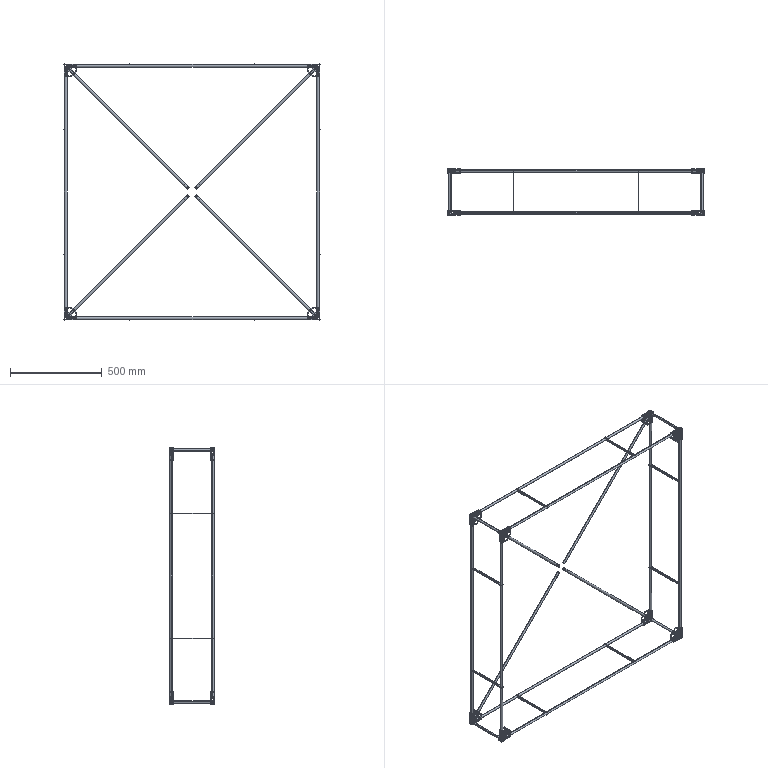Part | SolidWorks | 132 solids | 3392 faces | volume 484779 mm3 | cylinder 1880 | plane 1512 | commonest cylinder face diameters 3.1 x688 3 x416 6 x272 4 x112 14 x104 12 x40